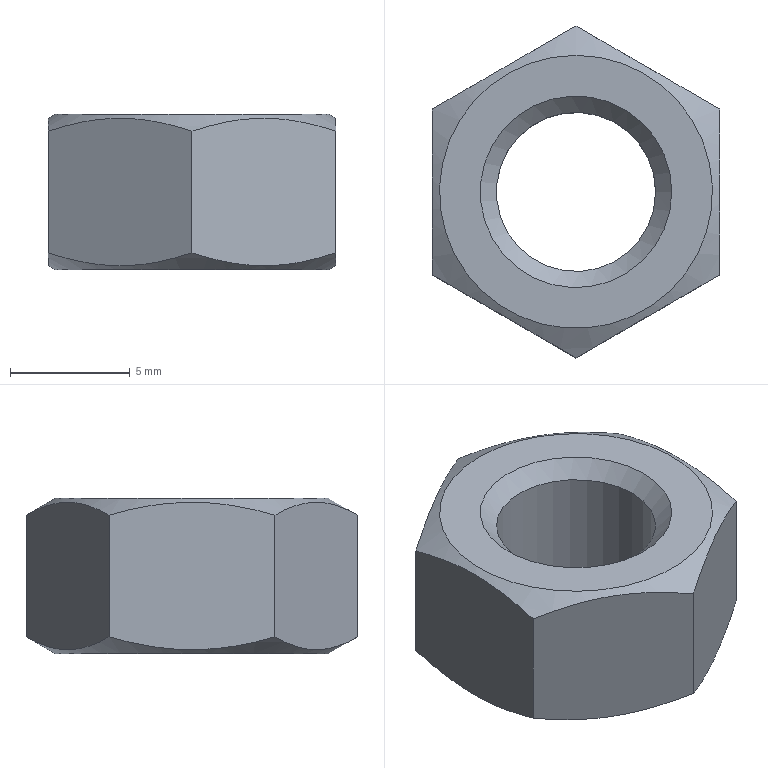Part | STEP file | Гайка М8-6H ГОСТ 15521-70 | 1 solid | 13 faces | box 12 x 13.856 x 6.5 mm | volume 565.148 mm3 | plane 8 | cone 4 | cylinder 1 | commonest cylinder face diameters 6.647 x1
STEP:
#1=CARTESIAN_POINT('',(0.,5.7,0.));
#2=VERTEX_POINT('',#1);
#3=CARTESIAN_POINT('',(0.,0.,0.));
#4=DIRECTION('',(0.,0.,-1.));
#5=DIRECTION('',(0.,1.,0.));
#6=AXIS2_PLACEMENT_3D('',#3,#4,#5);
#7=CIRCLE('',#6,5.7);
#8=EDGE_CURVE('',#2,#2,#7,.T.);
#9=ORIENTED_EDGE('',*,*,#8,.T.);
#10=EDGE_LOOP('',(#9));
#11=FACE_BOUND('',#10,.T.);
#12=CARTESIAN_POINT('',(4.,0.,0.));
#13=VERTEX_POINT('',#12);
#14=CARTESIAN_POINT('',(0.,0.,0.));
#15=DIRECTION('',(0.,0.,1.));
#16=DIRECTION('',(1.,0.,0.));
#17=AXIS2_PLACEMENT_3D('',#14,#15,#16);
#18=CIRCLE('',#17,4.);
#19=EDGE_CURVE('',#13,#13,#18,.T.);
#20=ORIENTED_EDGE('',*,*,#19,.T.);
#21=EDGE_LOOP('',(#20));
#22=FACE_BOUND('',#21,.T.);
#23=CARTESIAN_POINT('',(0.,0.,0.));
#24=DIRECTION('',(0.,0.,1.));
#25=DIRECTION('',(1.,0.,0.));
#26=AXIS2_PLACEMENT_3D('',#23,#24,#25);
#27=PLANE('',#26);
#28=ADVANCED_FACE('',(#11,#22),#27,.F.);
#29=CARTESIAN_POINT('',(-6.,3.464,0.7091));
#30=VERTEX_POINT('',#29);
#31=CARTESIAN_POINT('',(-6.,-3.464,0.7091));
#32=VERTEX_POINT('',#31);
#33=CARTESIAN_POINT('',(-6.,3.464,0.7091));
#34=CARTESIAN_POINT('',(-6.,3.44,0.7022));
#35=CARTESIAN_POINT('',(-6.,3.392,0.6884));
#36=CARTESIAN_POINT('',(-6.,3.319,0.6679));
#37=CARTESIAN_POINT('',(-6.,3.262,0.6521));
#38=CARTESIAN_POINT('',(-6.,3.212,0.6384));
#39=CARTESIAN_POINT('',(-6.,3.161,0.6244));
#40=CARTESIAN_POINT('',(-6.,3.081,0.6031));
#41=CARTESIAN_POINT('',(-6.,2.98,0.5769));
#42=CARTESIAN_POINT('',(-6.,2.867,0.5481));
#43=CARTESIAN_POINT('',(-6.,2.756,0.5211));
#44=CARTESIAN_POINT('',(-6.,2.667,0.4999));
#45=CARTESIAN_POINT('',(-6.,2.597,0.4838));
#46=CARTESIAN_POINT('',(-6.,2.519,0.4659));
#47=CARTESIAN_POINT('',(-6.,2.411,0.4423));
#48=CARTESIAN_POINT('',(-6.,2.271,0.4128));
#49=CARTESIAN_POINT('',(-6.,2.118,0.3823));
#50=CARTESIAN_POINT('',(-6.,1.93,0.3475));
#51=CARTESIAN_POINT('',(-6.,1.792,0.3241));
#52=CARTESIAN_POINT('',(-6.,1.624,0.2976));
#53=CARTESIAN_POINT('',(-6.,1.448,0.2716));
#54=CARTESIAN_POINT('',(-6.,1.203,0.2413));
#55=CARTESIAN_POINT('',(-6.,0.9715,0.2176));
#56=CARTESIAN_POINT('',(-6.,0.8175,0.2049));
#57=CARTESIAN_POINT('',(-6.,0.6729,0.1947));
#58=CARTESIAN_POINT('',(-6.,0.528,0.186));
#59=CARTESIAN_POINT('',(-6.,0.3241,0.1775));
#60=CARTESIAN_POINT('',(-6.,0.1444,0.1738));
#61=CARTESIAN_POINT('',(-6.,0.005553,0.173));
#62=CARTESIAN_POINT('',(-6.,-0.1288,0.1736));
#63=CARTESIAN_POINT('',(-6.,-0.2398,0.1757));
#64=CARTESIAN_POINT('',(-6.,-0.3697,0.1796));
#65=CARTESIAN_POINT('',(-6.,-0.4967,0.1846));
#66=CARTESIAN_POINT('',(-6.,-0.6724,0.1943));
#67=CARTESIAN_POINT('',(-6.,-0.8597,0.208));
#68=CARTESIAN_POINT('',(-6.,-1.046,0.2249));
#69=CARTESIAN_POINT('',(-6.,-1.17,0.2382));
#70=CARTESIAN_POINT('',(-6.,-1.292,0.2525));
#71=CARTESIAN_POINT('',(-6.,-1.414,0.2676));
#72=CARTESIAN_POINT('',(-6.,-1.595,0.293));
#73=CARTESIAN_POINT('',(-6.,-1.774,0.321));
#74=CARTESIAN_POINT('',(-6.,-1.901,0.3428));
#75=CARTESIAN_POINT('',(-6.,-2.018,0.3638));
#76=CARTESIAN_POINT('',(-6.,-2.134,0.3855));
#77=CARTESIAN_POINT('',(-6.,-2.299,0.4185));
#78=CARTESIAN_POINT('',(-6.,-2.471,0.455));
#79=CARTESIAN_POINT('',(-6.,-2.64,0.4933));
#80=CARTESIAN_POINT('',(-6.,-2.785,0.528));
#81=CARTESIAN_POINT('',(-6.,-2.896,0.5556));
#82=CARTESIAN_POINT('',(-6.,-3.007,0.5836));
#83=CARTESIAN_POINT('',(-6.,-3.138,0.6181));
#84=CARTESIAN_POINT('',(-6.,-3.294,0.6607));
#85=CARTESIAN_POINT('',(-6.,-3.403,0.6914));
#86=CARTESIAN_POINT('',(-6.,-3.457,0.707));
#87=CARTESIAN_POINT('',(-6.,-3.464,0.7091));
#88=B_SPLINE_CURVE_WITH_KNOTS('',3,(#33,#34,#35,#36,#37,#38,#39,#40,#41,#42,#43,#44,#45,#46,#47,#48,#49,#50,#51,#52,#53,#54,#55,#56,#57,#58,#59,#60,#61,#62,#63,#64,#65,#66,#67,#68,#69,#70,#71,#72,#73,#74,#75,#76,#77,#78,#79,#80,#81,#82,#83,#84,#85,#86,#87),.UNSPECIFIED.,.F.,.F.,(4,1,1,1,1,1,1,1,1,1,1,1,1,1,1,1,1,1,1,1,1,1,1,1,1,1,1,1,1,1,1,1,1,1,1,1,1,1,1,1,1,1,1,1,1,1,1,1,1,1,1,1,4),(0.,0.01059,0.02135,0.03227,0.03583,0.04354,0.05498,0.07113,0.0878,0.105,0.1195,0.127,0.1355,0.154,0.1738,0.1965,0.2208,0.2552,0.2563,0.2931,0.3312,0.3616,0.3923,0.3971,0.4234,0.4542,0.4842,0.5,0.5134,0.5414,0.5473,0.5689,0.5957,0.6224,0.649,0.6754,0.6755,0.7016,0.7277,0.7534,0.779,0.7826,0.8042,0.8294,0.8542,0.8789,0.9033,0.918,0.9277,0.9518,0.976,0.9967,1.),.UNSPECIFIED.);
#89=EDGE_CURVE('',#30,#32,#88,.T.);
#90=ORIENTED_EDGE('',*,*,#89,.T.);
#91=CARTESIAN_POINT('',(-6.,-3.464,5.791));
#92=VERTEX_POINT('',#91);
#93=CARTESIAN_POINT('',(-6.,-3.464,0.7091));
#94=DIRECTION('',(0.,0.,1.));
#95=VECTOR('',#94,1.);
#96=LINE('',#93,#95);
#97=EDGE_CURVE('',#32,#92,#96,.T.);
#98=ORIENTED_EDGE('',*,*,#97,.T.);
#99=CARTESIAN_POINT('',(-6.,3.464,5.791));
#100=VERTEX_POINT('',#99);
#101=CARTESIAN_POINT('',(-6.,-3.464,5.791));
#102=CARTESIAN_POINT('',(-6.,-3.44,5.798));
#103=CARTESIAN_POINT('',(-6.,-3.392,5.812));
#104=CARTESIAN_POINT('',(-6.,-3.319,5.832));
#105=CARTESIAN_POINT('',(-6.,-3.262,5.848));
#106=CARTESIAN_POINT('',(-6.,-3.212,5.862));
#107=CARTESIAN_POINT('',(-6.,-3.161,5.876));
#108=CARTESIAN_POINT('',(-6.,-3.081,5.897));
#109=CARTESIAN_POINT('',(-6.,-2.98,5.923));
#110=CARTESIAN_POINT('',(-6.,-2.867,5.952));
#111=CARTESIAN_POINT('',(-6.,-2.756,5.979));
#112=CARTESIAN_POINT('',(-6.,-2.667,6.));
#113=CARTESIAN_POINT('',(-6.,-2.597,6.016));
#114=CARTESIAN_POINT('',(-6.,-2.519,6.034));
#115=CARTESIAN_POINT('',(-6.,-2.411,6.058));
#116=CARTESIAN_POINT('',(-6.,-2.271,6.087));
#117=CARTESIAN_POINT('',(-6.,-2.118,6.118));
#118=CARTESIAN_POINT('',(-6.,-1.93,6.153));
#119=CARTESIAN_POINT('',(-6.,-1.792,6.176));
#120=CARTESIAN_POINT('',(-6.,-1.624,6.202));
#121=CARTESIAN_POINT('',(-6.,-1.448,6.228));
#122=CARTESIAN_POINT('',(-6.,-1.203,6.259));
#123=CARTESIAN_POINT('',(-6.,-0.9715,6.282));
#124=CARTESIAN_POINT('',(-6.,-0.8175,6.295));
#125=CARTESIAN_POINT('',(-6.,-0.6729,6.305));
#126=CARTESIAN_POINT('',(-6.,-0.528,6.314));
#127=CARTESIAN_POINT('',(-6.,-0.3241,6.322));
#128=CARTESIAN_POINT('',(-6.,-0.1444,6.326));
#129=CARTESIAN_POINT('',(-6.,-0.005553,6.327));
#130=CARTESIAN_POINT('',(-6.,0.1288,6.326));
#131=CARTESIAN_POINT('',(-6.,0.2398,6.324));
#132=CARTESIAN_POINT('',(-6.,0.3697,6.32));
#133=CARTESIAN_POINT('',(-6.,0.4967,6.315));
#134=CARTESIAN_POINT('',(-6.,0.6724,6.306));
#135=CARTESIAN_POINT('',(-6.,0.8597,6.292));
#136=CARTESIAN_POINT('',(-6.,1.046,6.275));
#137=CARTESIAN_POINT('',(-6.,1.17,6.262));
#138=CARTESIAN_POINT('',(-6.,1.292,6.248));
#139=CARTESIAN_POINT('',(-6.,1.414,6.232));
#140=CARTESIAN_POINT('',(-6.,1.595,6.207));
#141=CARTESIAN_POINT('',(-6.,1.774,6.179));
#142=CARTESIAN_POINT('',(-6.,1.901,6.157));
#143=CARTESIAN_POINT('',(-6.,2.018,6.136));
#144=CARTESIAN_POINT('',(-6.,2.134,6.114));
#145=CARTESIAN_POINT('',(-6.,2.299,6.082));
#146=CARTESIAN_POINT('',(-6.,2.471,6.045));
#147=CARTESIAN_POINT('',(-6.,2.64,6.007));
#148=CARTESIAN_POINT('',(-6.,2.785,5.972));
#149=CARTESIAN_POINT('',(-6.,2.896,5.944));
#150=CARTESIAN_POINT('',(-6.,3.007,5.916));
#151=CARTESIAN_POINT('',(-6.,3.138,5.882));
#152=CARTESIAN_POINT('',(-6.,3.294,5.839));
#153=CARTESIAN_POINT('',(-6.,3.403,5.809));
#154=CARTESIAN_POINT('',(-6.,3.457,5.793));
#155=CARTESIAN_POINT('',(-6.,3.464,5.791));
#156=B_SPLINE_CURVE_WITH_KNOTS('',3,(#101,#102,#103,#104,#105,#106,#107,#108,#109,#110,#111,#112,#113,#114,#115,#116,#117,#118,#119,#120,#121,#122,#123,#124,#125,#126,#127,#128,#129,#130,#131,#132,#133,#134,#135,#136,#137,#138,#139,#140,#141,#142,#143,#144,#145,#146,#147,#148,#149,#150,#151,#152,#153,#154,#155),.UNSPECIFIED.,.F.,.F.,(4,1,1,1,1,1,1,1,1,1,1,1,1,1,1,1,1,1,1,1,1,1,1,1,1,1,1,1,1,1,1,1,1,1,1,1,1,1,1,1,1,1,1,1,1,1,1,1,1,1,1,1,4),(0.,0.01059,0.02135,0.03227,0.03583,0.04354,0.05498,0.07113,0.0878,0.105,0.1195,0.127,0.1355,0.154,0.1738,0.1965,0.2208,0.2552,0.2563,0.2931,0.3312,0.3616,0.3923,0.3971,0.4234,0.4542,0.4842,0.5,0.5134,0.5414,0.5473,0.5689,0.5957,0.6224,0.649,0.6754,0.6755,0.7016,0.7277,0.7534,0.779,0.7826,0.8042,0.8294,0.8542,0.8789,0.9033,0.918,0.9277,0.9518,0.976,0.9967,1.),.UNSPECIFIED.);
#157=EDGE_CURVE('',#92,#100,#156,.T.);
#158=ORIENTED_EDGE('',*,*,#157,.T.);
#159=CARTESIAN_POINT('',(-6.,3.464,0.7091));
#160=DIRECTION('',(0.,0.,1.));
#161=VECTOR('',#160,1.);
#162=LINE('',#159,#161);
#163=EDGE_CURVE('',#30,#100,#162,.T.);
#164=ORIENTED_EDGE('',*,*,#163,.F.);
#165=EDGE_LOOP('',(#90,#98,#158,#164));
#166=FACE_BOUND('',#165,.T.);
#167=CARTESIAN_POINT('',(-6.,3.464,0.));
#168=DIRECTION('',(-1.,0.,0.));
#169=DIRECTION('',(0.,-1.,0.));
#170=AXIS2_PLACEMENT_3D('',#167,#168,#169);
#171=PLANE('',#170);
#172=ADVANCED_FACE('',(#166),#171,.T.);
#173=CARTESIAN_POINT('',(0.,6.928,0.7091));
#174=VERTEX_POINT('',#173);
#175=CARTESIAN_POINT('',(0.,6.928,0.7091));
#176=CARTESIAN_POINT('',(-0.02065,6.916,0.7022));
#177=CARTESIAN_POINT('',(-0.06231,6.892,0.6884));
#178=CARTESIAN_POINT('',(-0.1254,6.856,0.6679));
#179=CARTESIAN_POINT('',(-0.1899,6.819,0.6473));
#180=CARTESIAN_POINT('',(-0.2557,6.781,0.6266));
#181=CARTESIAN_POINT('',(-0.332,6.737,0.6031));
#182=CARTESIAN_POINT('',(-0.419,6.686,0.5769));
#183=CARTESIAN_POINT('',(-0.5174,6.629,0.5481));
#184=CARTESIAN_POINT('',(-0.6129,6.574,0.5211));
#185=CARTESIAN_POINT('',(-0.7071,6.52,0.4954));
#186=CARTESIAN_POINT('',(-0.8041,6.464,0.4697));
#187=CARTESIAN_POINT('',(-0.9117,6.402,0.4423));
#188=CARTESIAN_POINT('',(-1.033,6.332,0.4128));
#189=CARTESIAN_POINT('',(-1.166,6.255,0.3823));
#190=CARTESIAN_POINT('',(-1.331,6.16,0.347));
#191=CARTESIAN_POINT('',(-1.524,6.048,0.3093));
#192=CARTESIAN_POINT('',(-1.746,5.92,0.2716));
#193=CARTESIAN_POINT('',(-1.958,5.798,0.2413));
#194=CARTESIAN_POINT('',(-2.159,5.682,0.2176));
#195=CARTESIAN_POINT('',(-2.345,5.574,0.1999));
#196=CARTESIAN_POINT('',(-2.533,5.466,0.1864));
#197=CARTESIAN_POINT('',(-2.719,5.358,0.1775));
#198=CARTESIAN_POINT('',(-2.875,5.268,0.1738));
#199=CARTESIAN_POINT('',(-2.995,5.199,0.173));
#200=CARTESIAN_POINT('',(-3.112,5.132,0.1736));
#201=CARTESIAN_POINT('',(-3.251,5.051,0.1766));
#202=CARTESIAN_POINT('',(-3.418,4.955,0.1838));
#203=CARTESIAN_POINT('',(-3.582,4.86,0.1943));
#204=CARTESIAN_POINT('',(-3.745,4.766,0.208));
#205=CARTESIAN_POINT('',(-3.906,4.673,0.2249));
#206=CARTESIAN_POINT('',(-4.066,4.581,0.2448));
#207=CARTESIAN_POINT('',(-4.224,4.489,0.2676));
#208=CARTESIAN_POINT('',(-4.381,4.399,0.293));
#209=CARTESIAN_POINT('',(-4.536,4.309,0.321));
#210=CARTESIAN_POINT('',(-4.69,4.221,0.3513));
#211=CARTESIAN_POINT('',(-4.841,4.133,0.3839));
#212=CARTESIAN_POINT('',(-4.991,4.047,0.4185));
#213=CARTESIAN_POINT('',(-5.14,3.961,0.455));
#214=CARTESIAN_POINT('',(-5.286,3.876,0.4933));
#215=CARTESIAN_POINT('',(-5.431,3.792,0.5333));
#216=CARTESIAN_POINT('',(-5.575,3.709,0.5749));
#217=CARTESIAN_POINT('',(-5.718,3.627,0.6181));
#218=CARTESIAN_POINT('',(-5.859,3.545,0.6627));
#219=CARTESIAN_POINT('',(-5.953,3.491,0.6935));
#220=CARTESIAN_POINT('',(-6.,3.464,0.7091));
#221=B_SPLINE_CURVE_WITH_KNOTS('',3,(#175,#176,#177,#178,#179,#180,#181,#182,#183,#184,#185,#186,#187,#188,#189,#190,#191,#192,#193,#194,#195,#196,#197,#198,#199,#200,#201,#202,#203,#204,#205,#206,#207,#208,#209,#210,#211,#212,#213,#214,#215,#216,#217,#218,#219,#220),.UNSPECIFIED.,.F.,.F.,(4,1,1,1,1,1,1,1,1,1,1,1,1,1,1,1,1,1,1,1,1,1,1,1,1,1,1,1,1,1,1,1,1,1,1,1,1,1,1,1,1,1,1,4),(0.,0.01059,0.02135,0.03227,0.04354,0.05498,0.07113,0.0878,0.105,0.1195,0.1355,0.154,0.1738,0.1965,0.2208,0.2563,0.2931,0.3312,0.3616,0.3923,0.4234,0.4542,0.4842,0.5,0.5134,0.5414,0.5689,0.5957,0.6224,0.649,0.6754,0.7016,0.7277,0.7534,0.779,0.8042,0.8294,0.8542,0.8789,0.9033,0.9277,0.9518,0.976,1.),.UNSPECIFIED.);
#222=EDGE_CURVE('',#174,#30,#221,.T.);
#223=ORIENTED_EDGE('',*,*,#222,.T.);
#224=ORIENTED_EDGE('',*,*,#163,.T.);
#225=CARTESIAN_POINT('',(0.,6.928,5.791));
#226=VERTEX_POINT('',#225);
#227=CARTESIAN_POINT('',(-6.,3.464,5.791));
#228=CARTESIAN_POINT('',(-5.979,3.476,5.798));
#229=CARTESIAN_POINT('',(-5.938,3.5,5.812));
#230=CARTESIAN_POINT('',(-5.875,3.536,5.832));
#231=CARTESIAN_POINT('',(-5.81,3.574,5.853));
#232=CARTESIAN_POINT('',(-5.744,3.612,5.873));
#233=CARTESIAN_POINT('',(-5.668,3.656,5.897));
#234=CARTESIAN_POINT('',(-5.581,3.706,5.923));
#235=CARTESIAN_POINT('',(-5.483,3.763,5.952));
#236=CARTESIAN_POINT('',(-5.387,3.818,5.979));
#237=CARTESIAN_POINT('',(-5.293,3.872,6.005));
#238=CARTESIAN_POINT('',(-5.196,3.928,6.03));
#239=CARTESIAN_POINT('',(-5.088,3.99,6.058));
#240=CARTESIAN_POINT('',(-4.967,4.06,6.087));
#241=CARTESIAN_POINT('',(-4.834,4.137,6.118));
#242=CARTESIAN_POINT('',(-4.669,4.232,6.153));
#243=CARTESIAN_POINT('',(-4.476,4.344,6.191));
#244=CARTESIAN_POINT('',(-4.254,4.472,6.228));
#245=CARTESIAN_POINT('',(-4.042,4.595,6.259));
#246=CARTESIAN_POINT('',(-3.841,4.71,6.282));
#247=CARTESIAN_POINT('',(-3.655,4.818,6.3));
#248=CARTESIAN_POINT('',(-3.467,4.927,6.314));
#249=CARTESIAN_POINT('',(-3.281,5.034,6.322));
#250=CARTESIAN_POINT('',(-3.125,5.124,6.326));
#251=CARTESIAN_POINT('',(-3.005,5.193,6.327));
#252=CARTESIAN_POINT('',(-2.888,5.261,6.326));
#253=CARTESIAN_POINT('',(-2.749,5.341,6.323));
#254=CARTESIAN_POINT('',(-2.582,5.438,6.316));
#255=CARTESIAN_POINT('',(-2.418,5.532,6.306));
#256=CARTESIAN_POINT('',(-2.255,5.626,6.292));
#257=CARTESIAN_POINT('',(-2.094,5.719,6.275));
#258=CARTESIAN_POINT('',(-1.934,5.811,6.255));
#259=CARTESIAN_POINT('',(-1.776,5.903,6.232));
#260=CARTESIAN_POINT('',(-1.619,5.994,6.207));
#261=CARTESIAN_POINT('',(-1.464,6.083,6.179));
#262=CARTESIAN_POINT('',(-1.31,6.172,6.149));
#263=CARTESIAN_POINT('',(-1.159,6.259,6.116));
#264=CARTESIAN_POINT('',(-1.009,6.346,6.082));
#265=CARTESIAN_POINT('',(-0.8604,6.431,6.045));
#266=CARTESIAN_POINT('',(-0.7138,6.516,6.007));
#267=CARTESIAN_POINT('',(-0.5687,6.6,5.967));
#268=CARTESIAN_POINT('',(-0.425,6.683,5.925));
#269=CARTESIAN_POINT('',(-0.2824,6.765,5.882));
#270=CARTESIAN_POINT('',(-0.1408,6.847,5.837));
#271=CARTESIAN_POINT('',(-0.04683,6.901,5.807));
#272=CARTESIAN_POINT('',(0.000000002,6.928,5.791));
#273=B_SPLINE_CURVE_WITH_KNOTS('',3,(#227,#228,#229,#230,#231,#232,#233,#234,#235,#236,#237,#238,#239,#240,#241,#242,#243,#244,#245,#246,#247,#248,#249,#250,#251,#252,#253,#254,#255,#256,#257,#258,#259,#260,#261,#262,#263,#264,#265,#266,#267,#268,#269,#270,#271,#272),.UNSPECIFIED.,.F.,.F.,(4,1,1,1,1,1,1,1,1,1,1,1,1,1,1,1,1,1,1,1,1,1,1,1,1,1,1,1,1,1,1,1,1,1,1,1,1,1,1,1,1,1,1,4),(0.,0.01059,0.02135,0.03227,0.04354,0.05498,0.07113,0.0878,0.105,0.1195,0.1355,0.154,0.1738,0.1965,0.2208,0.2563,0.2931,0.3312,0.3616,0.3923,0.4234,0.4542,0.4842,0.5,0.5134,0.5414,0.5689,0.5957,0.6224,0.649,0.6754,0.7016,0.7277,0.7534,0.779,0.8042,0.8294,0.8542,0.8789,0.9033,0.9277,0.9518,0.976,1.),.UNSPECIFIED.);
#274=EDGE_CURVE('',#100,#226,#273,.T.);
#275=ORIENTED_EDGE('',*,*,#274,.T.);
#276=CARTESIAN_POINT('',(0.,6.928,0.7091));
#277=DIRECTION('',(0.,0.,1.));
#278=VECTOR('',#277,1.);
#279=LINE('',#276,#278);
#280=EDGE_CURVE('',#174,#226,#279,.T.);
#281=ORIENTED_EDGE('',*,*,#280,.F.);
#282=EDGE_LOOP('',(#223,#224,#275,#281));
#283=FACE_BOUND('',#282,.T.);
#284=CARTESIAN_POINT('',(0.,6.928,0.));
#285=DIRECTION('',(-0.5,0.866,0.));
#286=DIRECTION('',(-0.866,-0.5,0.));
#287=AXIS2_PLACEMENT_3D('',#284,#285,#286);
#288=PLANE('',#287);
#289=ADVANCED_FACE('',(#283),#288,.T.);
#290=CARTESIAN_POINT('',(6.,3.464,0.7091));
#291=VERTEX_POINT('',#290);
#292=CARTESIAN_POINT('',(6.,3.464,0.7091));
#293=CARTESIAN_POINT('',(5.979,3.476,0.7022));
#294=CARTESIAN_POINT('',(5.938,3.5,0.6884));
#295=CARTESIAN_POINT('',(5.875,3.536,0.6679));
#296=CARTESIAN_POINT('',(5.81,3.574,0.6473));
#297=CARTESIAN_POINT('',(5.744,3.612,0.6266));
#298=CARTESIAN_POINT('',(5.668,3.656,0.6031));
#299=CARTESIAN_POINT('',(5.581,3.706,0.5769));
#300=CARTESIAN_POINT('',(5.483,3.763,0.5481));
#301=CARTESIAN_POINT('',(5.387,3.818,0.5211));
#302=CARTESIAN_POINT('',(5.293,3.872,0.4954));
#303=CARTESIAN_POINT('',(5.196,3.928,0.4697));
#304=CARTESIAN_POINT('',(5.088,3.99,0.4423));
#305=CARTESIAN_POINT('',(4.967,4.06,0.4128));
#306=CARTESIAN_POINT('',(4.834,4.137,0.3823));
#307=CARTESIAN_POINT('',(4.669,4.232,0.347));
#308=CARTESIAN_POINT('',(4.476,4.344,0.3093));
#309=CARTESIAN_POINT('',(4.254,4.472,0.2716));
#310=CARTESIAN_POINT('',(4.042,4.595,0.2413));
#311=CARTESIAN_POINT('',(3.841,4.71,0.2176));
#312=CARTESIAN_POINT('',(3.655,4.818,0.1999));
#313=CARTESIAN_POINT('',(3.467,4.927,0.1864));
#314=CARTESIAN_POINT('',(3.281,5.034,0.1775));
#315=CARTESIAN_POINT('',(3.125,5.124,0.1738));
#316=CARTESIAN_POINT('',(3.005,5.193,0.173));
#317=CARTESIAN_POINT('',(2.888,5.261,0.1736));
#318=CARTESIAN_POINT('',(2.749,5.341,0.1766));
#319=CARTESIAN_POINT('',(2.582,5.438,0.1838));
#320=CARTESIAN_POINT('',(2.418,5.532,0.1943));
#321=CARTESIAN_POINT('',(2.255,5.626,0.208));
#322=CARTESIAN_POINT('',(2.094,5.719,0.2249));
#323=CARTESIAN_POINT('',(1.934,5.811,0.2448));
#324=CARTESIAN_POINT('',(1.776,5.903,0.2676));
#325=CARTESIAN_POINT('',(1.619,5.994,0.293));
#326=CARTESIAN_POINT('',(1.464,6.083,0.321));
#327=CARTESIAN_POINT('',(1.31,6.172,0.3513));
#328=CARTESIAN_POINT('',(1.159,6.259,0.3839));
#329=CARTESIAN_POINT('',(1.009,6.346,0.4185));
#330=CARTESIAN_POINT('',(0.8604,6.431,0.455));
#331=CARTESIAN_POINT('',(0.7138,6.516,0.4933));
#332=CARTESIAN_POINT('',(0.5687,6.6,0.5333));
#333=CARTESIAN_POINT('',(0.425,6.683,0.5749));
#334=CARTESIAN_POINT('',(0.2824,6.765,0.6181));
#335=CARTESIAN_POINT('',(0.1408,6.847,0.6627));
#336=CARTESIAN_POINT('',(0.04683,6.901,0.6935));
#337=CARTESIAN_POINT('',(0.000000002,6.928,0.7091));
#338=B_SPLINE_CURVE_WITH_KNOTS('',3,(#292,#293,#294,#295,#296,#297,#298,#299,#300,#301,#302,#303,#304,#305,#306,#307,#308,#309,#310,#311,#312,#313,#314,#315,#316,#317,#318,#319,#320,#321,#322,#323,#324,#325,#326,#327,#328,#329,#330,#331,#332,#333,#334,#335,#336,#337),.UNSPECIFIED.,.F.,.F.,(4,1,1,1,1,1,1,1,1,1,1,1,1,1,1,1,1,1,1,1,1,1,1,1,1,1,1,1,1,1,1,1,1,1,1,1,1,1,1,1,1,1,1,4),(0.,0.01059,0.02135,0.03227,0.04354,0.05498,0.07113,0.0878,0.105,0.1195,0.1355,0.154,0.1738,0.1965,0.2208,0.2563,0.2931,0.3312,0.3616,0.3923,0.4234,0.4542,0.4842,0.5,0.5134,0.5414,0.5689,0.5957,0.6224,0.649,0.6754,0.7016,0.7277,0.7534,0.779,0.8042,0.8294,0.8542,0.8789,0.9033,0.9277,0.9518,0.976,1.),.UNSPECIFIED.);
#339=EDGE_CURVE('',#291,#174,#338,.T.);
#340=ORIENTED_EDGE('',*,*,#339,.T.);
#341=ORIENTED_EDGE('',*,*,#280,.T.);
#342=CARTESIAN_POINT('',(6.,3.464,5.791));
#343=VERTEX_POINT('',#342);
#344=CARTESIAN_POINT('',(0.,6.928,5.791));
#345=CARTESIAN_POINT('',(0.02065,6.916,5.798));
#346=CARTESIAN_POINT('',(0.06231,6.892,5.812));
#347=CARTESIAN_POINT('',(0.1254,6.856,5.832));
#348=CARTESIAN_POINT('',(0.1899,6.819,5.853));
#349=CARTESIAN_POINT('',(0.2557,6.781,5.873));
#350=CARTESIAN_POINT('',(0.332,6.737,5.897));
#351=CARTESIAN_POINT('',(0.419,6.686,5.923));
#352=CARTESIAN_POINT('',(0.5174,6.629,5.952));
#353=CARTESIAN_POINT('',(0.6129,6.574,5.979));
#354=CARTESIAN_POINT('',(0.7071,6.52,6.005));
#355=CARTESIAN_POINT('',(0.8041,6.464,6.03));
#356=CARTESIAN_POINT('',(0.9117,6.402,6.058));
#357=CARTESIAN_POINT('',(1.033,6.332,6.087));
#358=CARTESIAN_POINT('',(1.166,6.255,6.118));
#359=CARTESIAN_POINT('',(1.331,6.16,6.153));
#360=CARTESIAN_POINT('',(1.524,6.048,6.191));
#361=CARTESIAN_POINT('',(1.746,5.92,6.228));
#362=CARTESIAN_POINT('',(1.958,5.798,6.259));
#363=CARTESIAN_POINT('',(2.159,5.682,6.282));
#364=CARTESIAN_POINT('',(2.345,5.574,6.3));
#365=CARTESIAN_POINT('',(2.533,5.466,6.314));
#366=CARTESIAN_POINT('',(2.719,5.358,6.322));
#367=CARTESIAN_POINT('',(2.875,5.268,6.326));
#368=CARTESIAN_POINT('',(2.995,5.199,6.327));
#369=CARTESIAN_POINT('',(3.112,5.132,6.326));
#370=CARTESIAN_POINT('',(3.251,5.051,6.323));
#371=CARTESIAN_POINT('',(3.418,4.955,6.316));
#372=CARTESIAN_POINT('',(3.582,4.86,6.306));
#373=CARTESIAN_POINT('',(3.745,4.766,6.292));
#374=CARTESIAN_POINT('',(3.906,4.673,6.275));
#375=CARTESIAN_POINT('',(4.066,4.581,6.255));
#376=CARTESIAN_POINT('',(4.224,4.489,6.232));
#377=CARTESIAN_POINT('',(4.381,4.399,6.207));
#378=CARTESIAN_POINT('',(4.536,4.309,6.179));
#379=CARTESIAN_POINT('',(4.69,4.221,6.149));
#380=CARTESIAN_POINT('',(4.841,4.133,6.116));
#381=CARTESIAN_POINT('',(4.991,4.047,6.082));
#382=CARTESIAN_POINT('',(5.14,3.961,6.045));
#383=CARTESIAN_POINT('',(5.286,3.876,6.007));
#384=CARTESIAN_POINT('',(5.431,3.792,5.967));
#385=CARTESIAN_POINT('',(5.575,3.709,5.925));
#386=CARTESIAN_POINT('',(5.718,3.627,5.882));
#387=CARTESIAN_POINT('',(5.859,3.545,5.837));
#388=CARTESIAN_POINT('',(5.953,3.491,5.807));
#389=CARTESIAN_POINT('',(6.,3.464,5.791));
#390=B_SPLINE_CURVE_WITH_KNOTS('',3,(#344,#345,#346,#347,#348,#349,#350,#351,#352,#353,#354,#355,#356,#357,#358,#359,#360,#361,#362,#363,#364,#365,#366,#367,#368,#369,#370,#371,#372,#373,#374,#375,#376,#377,#378,#379,#380,#381,#382,#383,#384,#385,#386,#387,#388,#389),.UNSPECIFIED.,.F.,.F.,(4,1,1,1,1,1,1,1,1,1,1,1,1,1,1,1,1,1,1,1,1,1,1,1,1,1,1,1,1,1,1,1,1,1,1,1,1,1,1,1,1,1,1,4),(0.,0.01059,0.02135,0.03227,0.04354,0.05498,0.07113,0.0878,0.105,0.1195,0.1355,0.154,0.1738,0.1965,0.2208,0.2563,0.2931,0.3312,0.3616,0.3923,0.4234,0.4542,0.4842,0.5,0.5134,0.5414,0.5689,0.5957,0.6224,0.649,0.6754,0.7016,0.7277,0.7534,0.779,0.8042,0.8294,0.8542,0.8789,0.9033,0.9277,0.9518,0.976,1.),.UNSPECIFIED.);
#391=EDGE_CURVE('',#226,#343,#390,.T.);
#392=ORIENTED_EDGE('',*,*,#391,.T.);
#393=CARTESIAN_POINT('',(6.,3.464,0.7091));
#394=DIRECTION('',(0.,0.,1.));
#395=VECTOR('',#394,1.);
#396=LINE('',#393,#395);
#397=EDGE_CURVE('',#291,#343,#396,.T.);
#398=ORIENTED_EDGE('',*,*,#397,.F.);
#399=EDGE_LOOP('',(#340,#341,#392,#398));
#400=FACE_BOUND('',#399,.T.);
#401=CARTESIAN_POINT('',(6.,3.464,0.));
#402=DIRECTION('',(0.5,0.866,0.));
#403=DIRECTION('',(-0.866,0.5,0.));
#404=AXIS2_PLACEMENT_3D('',#401,#402,#403);
#405=PLANE('',#404);
#406=ADVANCED_FACE('',(#400),#405,.T.);
#407=CARTESIAN_POINT('',(6.,-3.464,0.7091));
#408=VERTEX_POINT('',#407);
#409=CARTESIAN_POINT('',(6.,-3.464,0.7091));
#410=CARTESIAN_POINT('',(6.,-3.44,0.7022));
#411=CARTESIAN_POINT('',(6.,-3.392,0.6884));
#412=CARTESIAN_POINT('',(6.,-3.319,0.6679));
#413=CARTESIAN_POINT('',(6.,-3.262,0.6521));
#414=CARTESIAN_POINT('',(6.,-3.212,0.6384));
#415=CARTESIAN_POINT('',(6.,-3.161,0.6244));
#416=CARTESIAN_POINT('',(6.,-3.081,0.6031));
#417=CARTESIAN_POINT('',(6.,-2.98,0.5769));
#418=CARTESIAN_POINT('',(6.,-2.867,0.5481));
#419=CARTESIAN_POINT('',(6.,-2.756,0.5211));
#420=CARTESIAN_POINT('',(6.,-2.667,0.4999));
#421=CARTESIAN_POINT('',(6.,-2.597,0.4838));
#422=CARTESIAN_POINT('',(6.,-2.519,0.4659));
#423=CARTESIAN_POINT('',(6.,-2.411,0.4423));
#424=CARTESIAN_POINT('',(6.,-2.271,0.4128));
#425=CARTESIAN_POINT('',(6.,-2.118,0.3823));
#426=CARTESIAN_POINT('',(6.,-1.93,0.3475));
#427=CARTESIAN_POINT('',(6.,-1.792,0.3241));
#428=CARTESIAN_POINT('',(6.,-1.624,0.2976));
#429=CARTESIAN_POINT('',(6.,-1.448,0.2716));
#430=CARTESIAN_POINT('',(6.,-1.203,0.2413));
#431=CARTESIAN_POINT('',(6.,-0.9715,0.2176));
#432=CARTESIAN_POINT('',(6.,-0.8175,0.2049));
#433=CARTESIAN_POINT('',(6.,-0.6729,0.1947));
#434=CARTESIAN_POINT('',(6.,-0.528,0.186));
#435=CARTESIAN_POINT('',(6.,-0.3241,0.1775));
#436=CARTESIAN_POINT('',(6.,-0.1444,0.1738));
#437=CARTESIAN_POINT('',(6.,-0.005553,0.173));
#438=CARTESIAN_POINT('',(6.,0.1288,0.1736));
#439=CARTESIAN_POINT('',(6.,0.2398,0.1757));
#440=CARTESIAN_POINT('',(6.,0.3697,0.1796));
#441=CARTESIAN_POINT('',(6.,0.4967,0.1846));
#442=CARTESIAN_POINT('',(6.,0.6724,0.1943));
#443=CARTESIAN_POINT('',(6.,0.8597,0.208));
#444=CARTESIAN_POINT('',(6.,1.046,0.2249));
#445=CARTESIAN_POINT('',(6.,1.17,0.2382));
#446=CARTESIAN_POINT('',(6.,1.292,0.2525));
#447=CARTESIAN_POINT('',(6.,1.414,0.2676));
#448=CARTESIAN_POINT('',(6.,1.595,0.293));
#449=CARTESIAN_POINT('',(6.,1.774,0.321));
#450=CARTESIAN_POINT('',(6.,1.901,0.3428));
#451=CARTESIAN_POINT('',(6.,2.018,0.3638));
#452=CARTESIAN_POINT('',(6.,2.134,0.3855));
#453=CARTESIAN_POINT('',(6.,2.299,0.4185));
#454=CARTESIAN_POINT('',(6.,2.471,0.455));
#455=CARTESIAN_POINT('',(6.,2.64,0.4933));
#456=CARTESIAN_POINT('',(6.,2.785,0.528));
#457=CARTESIAN_POINT('',(6.,2.896,0.5556));
#458=CARTESIAN_POINT('',(6.,3.007,0.5836));
#459=CARTESIAN_POINT('',(6.,3.138,0.6181));
#460=CARTESIAN_POINT('',(6.,3.294,0.6607));
#461=CARTESIAN_POINT('',(6.,3.403,0.6914));
#462=CARTESIAN_POINT('',(6.,3.457,0.707));
#463=CARTESIAN_POINT('',(6.,3.464,0.7091));
#464=B_SPLINE_CURVE_WITH_KNOTS('',3,(#409,#410,#411,#412,#413,#414,#415,#416,#417,#418,#419,#420,#421,#422,#423,#424,#425,#426,#427,#428,#429,#430,#431,#432,#433,#434,#435,#436,#437,#438,#439,#440,#441,#442,#443,#444,#445,#446,#447,#448,#449,#450,#451,#452,#453,#454,#455,#456,#457,#458,#459,#460,#461,#462,#463),.UNSPECIFIED.,.F.,.F.,(4,1,1,1,1,1,1,1,1,1,1,1,1,1,1,1,1,1,1,1,1,1,1,1,1,1,1,1,1,1,1,1,1,1,1,1,1,1,1,1,1,1,1,1,1,1,1,1,1,1,1,1,4),(0.,0.01059,0.02135,0.03227,0.03583,0.04354,0.05498,0.07113,0.0878,0.105,0.1195,0.127,0.1355,0.154,0.1738,0.1965,0.2208,0.2552,0.2563,0.2931,0.3312,0.3616,0.3923,0.3971,0.4234,0.4542,0.4842,0.5,0.5134,0.5414,0.5473,0.5689,0.5957,0.6224,0.649,0.6754,0.6755,0.7016,0.7277,0.7534,0.779,0.7826,0.8042,0.8294,0.8542,0.8789,0.9033,0.918,0.9277,0.9518,0.976,0.9967,1.),.UNSPECIFIED.);
#465=EDGE_CURVE('',#408,#291,#464,.T.);
#466=ORIENTED_EDGE('',*,*,#465,.T.);
#467=ORIENTED_EDGE('',*,*,#397,.T.);
#468=CARTESIAN_POINT('',(6.,-3.464,5.791));
#469=VERTEX_POINT('',#468);
#470=CARTESIAN_POINT('',(6.,3.464,5.791));
#471=CARTESIAN_POINT('',(6.,3.44,5.798));
#472=CARTESIAN_POINT('',(6.,3.392,5.812));
#473=CARTESIAN_POINT('',(6.,3.319,5.832));
#474=CARTESIAN_POINT('',(6.,3.262,5.848));
#475=CARTESIAN_POINT('',(6.,3.212,5.862));
#476=CARTESIAN_POINT('',(6.,3.161,5.876));
#477=CARTESIAN_POINT('',(6.,3.081,5.897));
#478=CARTESIAN_POINT('',(6.,2.98,5.923));
#479=CARTESIAN_POINT('',(6.,2.867,5.952));
#480=CARTESIAN_POINT('',(6.,2.756,5.979));
#481=CARTESIAN_POINT('',(6.,2.667,6.));
#482=CARTESIAN_POINT('',(6.,2.597,6.016));
#483=CARTESIAN_POINT('',(6.,2.519,6.034));
#484=CARTESIAN_POINT('',(6.,2.411,6.058));
#485=CARTESIAN_POINT('',(6.,2.271,6.087));
#486=CARTESIAN_POINT('',(6.,2.118,6.118));
#487=CARTESIAN_POINT('',(6.,1.93,6.153));
#488=CARTESIAN_POINT('',(6.,1.792,6.176));
#489=CARTESIAN_POINT('',(6.,1.624,6.202));
#490=CARTESIAN_POINT('',(6.,1.448,6.228));
#491=CARTESIAN_POINT('',(6.,1.203,6.259));
#492=CARTESIAN_POINT('',(6.,0.9715,6.282));
#493=CARTESIAN_POINT('',(6.,0.8175,6.295));
#494=CARTESIAN_POINT('',(6.,0.6729,6.305));
#495=CARTESIAN_POINT('',(6.,0.528,6.314));
#496=CARTESIAN_POINT('',(6.,0.3241,6.322));
#497=CARTESIAN_POINT('',(6.,0.1444,6.326));
#498=CARTESIAN_POINT('',(6.,0.005553,6.327));
#499=CARTESIAN_POINT('',(6.,-0.1288,6.326));
#500=CARTESIAN_POINT('',(6.,-0.2398,6.324));
#501=CARTESIAN_POINT('',(6.,-0.3697,6.32));
#502=CARTESIAN_POINT('',(6.,-0.4967,6.315));
#503=CARTESIAN_POINT('',(6.,-0.6724,6.306));
#504=CARTESIAN_POINT('',(6.,-0.8597,6.292));
#505=CARTESIAN_POINT('',(6.,-1.046,6.275));
#506=CARTESIAN_POINT('',(6.,-1.17,6.262));
#507=CARTESIAN_POINT('',(6.,-1.292,6.248));
#508=CARTESIAN_POINT('',(6.,-1.414,6.232));
#509=CARTESIAN_POINT('',(6.,-1.595,6.207));
#510=CARTESIAN_POINT('',(6.,-1.774,6.179));
#511=CARTESIAN_POINT('',(6.,-1.901,6.157));
#512=CARTESIAN_POINT('',(6.,-2.018,6.136));
#513=CARTESIAN_POINT('',(6.,-2.134,6.114));
#514=CARTESIAN_POINT('',(6.,-2.299,6.082));
#515=CARTESIAN_POINT('',(6.,-2.471,6.045));
#516=CARTESIAN_POINT('',(6.,-2.64,6.007));
#517=CARTESIAN_POINT('',(6.,-2.785,5.972));
#518=CARTESIAN_POINT('',(6.,-2.896,5.944));
#519=CARTESIAN_POINT('',(6.,-3.007,5.916));
#520=CARTESIAN_POINT('',(6.,-3.138,5.882));
#521=CARTESIAN_POINT('',(6.,-3.294,5.839));
#522=CARTESIAN_POINT('',(6.,-3.403,5.809));
#523=CARTESIAN_POINT('',(6.,-3.457,5.793));
#524=CARTESIAN_POINT('',(6.,-3.464,5.791));
#525=B_SPLINE_CURVE_WITH_KNOTS('',3,(#470,#471,#472,#473,#474,#475,#476,#477,#478,#479,#480,#481,#482,#483,#484,#485,#486,#487,#488,#489,#490,#491,#492,#493,#494,#495,#496,#497,#498,#499,#500,#501,#502,#503,#504,#505,#506,#507,#508,#509,#510,#511,#512,#513,#514,#515,#516,#517,#518,#519,#520,#521,#522,#523,#524),.UNSPECIFIED.,.F.,.F.,(4,1,1,1,1,1,1,1,1,1,1,1,1,1,1,1,1,1,1,1,1,1,1,1,1,1,1,1,1,1,1,1,1,1,1,1,1,1,1,1,1,1,1,1,1,1,1,1,1,1,1,1,4),(0.,0.01059,0.02135,0.03227,0.03583,0.04354,0.05498,0.07113,0.0878,0.105,0.1195,0.127,0.1355,0.154,0.1738,0.1965,0.2208,0.2552,0.2563,0.2931,0.3312,0.3616,0.3923,0.3971,0.4234,0.4542,0.4842,0.5,0.5134,0.5414,0.5473,0.5689,0.5957,0.6224,0.649,0.6754,0.6755,0.7016,0.7277,0.7534,0.779,0.7826,0.8042,0.8294,0.8542,0.8789,0.9033,0.918,0.9277,0.9518,0.976,0.9967,1.),.UNSPECIFIED.);
#526=EDGE_CURVE('',#343,#469,#525,.T.);
#527=ORIENTED_EDGE('',*,*,#526,.T.);
#528=CARTESIAN_POINT('',(6.,-3.464,0.7091));
#529=DIRECTION('',(0.,0.,1.));
#530=VECTOR('',#529,1.);
#531=LINE('',#528,#530);
#532=EDGE_CURVE('',#408,#469,#531,.T.);
#533=ORIENTED_EDGE('',*,*,#532,.F.);
#534=EDGE_LOOP('',(#466,#467,#527,#533));
#535=FACE_BOUND('',#534,.T.);
#536=CARTESIAN_POINT('',(6.,-3.464,0.));
#537=DIRECTION('',(1.,0.,0.));
#538=DIRECTION('',(0.,1.,0.));
#539=AXIS2_PLACEMENT_3D('',#536,#537,#538);
#540=PLANE('',#539);
#541=ADVANCED_FACE('',(#535),#540,.T.);
#542=CARTESIAN_POINT('',(0.,-6.928,0.7091));
#543=VERTEX_POINT('',#542);
#544=CARTESIAN_POINT('',(0.,-6.928,0.7091));
#545=CARTESIAN_POINT('',(0.02065,-6.916,0.7022));
#546=CARTESIAN_POINT('',(0.06231,-6.892,0.6884));
#547=CARTESIAN_POINT('',(0.1254,-6.856,0.6679));
#548=CARTESIAN_POINT('',(0.1899,-6.819,0.6473));
#549=CARTESIAN_POINT('',(0.2557,-6.781,0.6266));
#550=CARTESIAN_POINT('',(0.332,-6.737,0.6031));
#551=CARTESIAN_POINT('',(0.419,-6.686,0.5769));
#552=CARTESIAN_POINT('',(0.5174,-6.629,0.5481));
#553=CARTESIAN_POINT('',(0.6129,-6.574,0.5211));
#554=CARTESIAN_POINT('',(0.7071,-6.52,0.4954));
#555=CARTESIAN_POINT('',(0.8041,-6.464,0.4697));
#556=CARTESIAN_POINT('',(0.9117,-6.402,0.4423));
#557=CARTESIAN_POINT('',(1.033,-6.332,0.4128));
#558=CARTESIAN_POINT('',(1.166,-6.255,0.3823));
#559=CARTESIAN_POINT('',(1.331,-6.16,0.347));
#560=CARTESIAN_POINT('',(1.524,-6.048,0.3093));
#561=CARTESIAN_POINT('',(1.746,-5.92,0.2716));
#562=CARTESIAN_POINT('',(1.958,-5.798,0.2413));
#563=CARTESIAN_POINT('',(2.159,-5.682,0.2176));
#564=CARTESIAN_POINT('',(2.345,-5.574,0.1999));
#565=CARTESIAN_POINT('',(2.533,-5.466,0.1864));
#566=CARTESIAN_POINT('',(2.719,-5.358,0.1775));
#567=CARTESIAN_POINT('',(2.875,-5.268,0.1738));
#568=CARTESIAN_POINT('',(2.995,-5.199,0.173));
#569=CARTESIAN_POINT('',(3.112,-5.132,0.1736));
#570=CARTESIAN_POINT('',(3.251,-5.051,0.1766));
#571=CARTESIAN_POINT('',(3.418,-4.955,0.1838));
#572=CARTESIAN_POINT('',(3.582,-4.86,0.1943));
#573=CARTESIAN_POINT('',(3.745,-4.766,0.208));
#574=CARTESIAN_POINT('',(3.906,-4.673,0.2249));
#575=CARTESIAN_POINT('',(4.066,-4.581,0.2448));
#576=CARTESIAN_POINT('',(4.224,-4.489,0.2676));
#577=CARTESIAN_POINT('',(4.381,-4.399,0.293));
#578=CARTESIAN_POINT('',(4.536,-4.309,0.321));
#579=CARTESIAN_POINT('',(4.69,-4.221,0.3513));
#580=CARTESIAN_POINT('',(4.841,-4.133,0.3839));
#581=CARTESIAN_POINT('',(4.991,-4.047,0.4185));
#582=CARTESIAN_POINT('',(5.14,-3.961,0.455));
#583=CARTESIAN_POINT('',(5.286,-3.876,0.4933));
#584=CARTESIAN_POINT('',(5.431,-3.792,0.5333));
#585=CARTESIAN_POINT('',(5.575,-3.709,0.5749));
#586=CARTESIAN_POINT('',(5.718,-3.627,0.6181));
#587=CARTESIAN_POINT('',(5.859,-3.545,0.6627));
#588=CARTESIAN_POINT('',(5.953,-3.491,0.6935));
#589=CARTESIAN_POINT('',(6.,-3.464,0.7091));
#590=B_SPLINE_CURVE_WITH_KNOTS('',3,(#544,#545,#546,#547,#548,#549,#550,#551,#552,#553,#554,#555,#556,#557,#558,#559,#560,#561,#562,#563,#564,#565,#566,#567,#568,#569,#570,#571,#572,#573,#574,#575,#576,#577,#578,#579,#580,#581,#582,#583,#584,#585,#586,#587,#588,#589),.UNSPECIFIED.,.F.,.F.,(4,1,1,1,1,1,1,1,1,1,1,1,1,1,1,1,1,1,1,1,1,1,1,1,1,1,1,1,1,1,1,1,1,1,1,1,1,1,1,1,1,1,1,4),(0.,0.01059,0.02135,0.03227,0.04354,0.05498,0.07113,0.0878,0.105,0.1195,0.1355,0.154,0.1738,0.1965,0.2208,0.2563,0.2931,0.3312,0.3616,0.3923,0.4234,0.4542,0.4842,0.5,0.5134,0.5414,0.5689,0.5957,0.6224,0.649,0.6754,0.7016,0.7277,0.7534,0.779,0.8042,0.8294,0.8542,0.8789,0.9033,0.9277,0.9518,0.976,1.),.UNSPECIFIED.);
#591=EDGE_CURVE('',#543,#408,#590,.T.);
#592=ORIENTED_EDGE('',*,*,#591,.T.);
#593=ORIENTED_EDGE('',*,*,#532,.T.);
#594=CARTESIAN_POINT('',(0.,-6.928,5.791));
#595=VERTEX_POINT('',#594);
#596=CARTESIAN_POINT('',(6.,-3.464,5.791));
#597=CARTESIAN_POINT('',(5.979,-3.476,5.798));
#598=CARTESIAN_POINT('',(5.938,-3.5,5.812));
#599=CARTESIAN_POINT('',(5.875,-3.536,5.832));
#600=CARTESIAN_POINT('',(5.81,-3.574,5.853));
#601=CARTESIAN_POINT('',(5.744,-3.612,5.873));
#602=CARTESIAN_POINT('',(5.668,-3.656,5.897));
#603=CARTESIAN_POINT('',(5.581,-3.706,5.923));
#604=CARTESIAN_POINT('',(5.483,-3.763,5.952));
#605=CARTESIAN_POINT('',(5.387,-3.818,5.979));
#606=CARTESIAN_POINT('',(5.293,-3.872,6.005));
#607=CARTESIAN_POINT('',(5.196,-3.928,6.03));
#608=CARTESIAN_POINT('',(5.088,-3.99,6.058));
#609=CARTESIAN_POINT('',(4.967,-4.06,6.087));
#610=CARTESIAN_POINT('',(4.834,-4.137,6.118));
#611=CARTESIAN_POINT('',(4.669,-4.232,6.153));
#612=CARTESIAN_POINT('',(4.476,-4.344,6.191));
#613=CARTESIAN_POINT('',(4.254,-4.472,6.228));
#614=CARTESIAN_POINT('',(4.042,-4.595,6.259));
#615=CARTESIAN_POINT('',(3.841,-4.71,6.282));
#616=CARTESIAN_POINT('',(3.655,-4.818,6.3));
#617=CARTESIAN_POINT('',(3.467,-4.927,6.314));
#618=CARTESIAN_POINT('',(3.281,-5.034,6.322));
#619=CARTESIAN_POINT('',(3.125,-5.124,6.326));
#620=CARTESIAN_POINT('',(3.005,-5.193,6.327));
#621=CARTESIAN_POINT('',(2.888,-5.261,6.326));
#622=CARTESIAN_POINT('',(2.749,-5.341,6.323));
#623=CARTESIAN_POINT('',(2.582,-5.438,6.316));
#624=CARTESIAN_POINT('',(2.418,-5.532,6.306));
#625=CARTESIAN_POINT('',(2.255,-5.626,6.292));
#626=CARTESIAN_POINT('',(2.094,-5.719,6.275));
#627=CARTESIAN_POINT('',(1.934,-5.811,6.255));
#628=CARTESIAN_POINT('',(1.776,-5.903,6.232));
#629=CARTESIAN_POINT('',(1.619,-5.994,6.207));
#630=CARTESIAN_POINT('',(1.464,-6.083,6.179));
#631=CARTESIAN_POINT('',(1.31,-6.172,6.149));
#632=CARTESIAN_POINT('',(1.159,-6.259,6.116));
#633=CARTESIAN_POINT('',(1.009,-6.346,6.082));
#634=CARTESIAN_POINT('',(0.8604,-6.431,6.045));
#635=CARTESIAN_POINT('',(0.7138,-6.516,6.007));
#636=CARTESIAN_POINT('',(0.5687,-6.6,5.967));
#637=CARTESIAN_POINT('',(0.425,-6.683,5.925));
#638=CARTESIAN_POINT('',(0.2824,-6.765,5.882));
#639=CARTESIAN_POINT('',(0.1408,-6.847,5.837));
#640=CARTESIAN_POINT('',(0.04683,-6.901,5.807));
#641=CARTESIAN_POINT('',(0.000000003,-6.928,5.791));
#642=B_SPLINE_CURVE_WITH_KNOTS('',3,(#596,#597,#598,#599,#600,#601,#602,#603,#604,#605,#606,#607,#608,#609,#610,#611,#612,#613,#614,#615,#616,#617,#618,#619,#620,#621,#622,#623,#624,#625,#626,#627,#628,#629,#630,#631,#632,#633,#634,#635,#636,#637,#638,#639,#640,#641),.UNSPECIFIED.,.F.,.F.,(4,1,1,1,1,1,1,1,1,1,1,1,1,1,1,1,1,1,1,1,1,1,1,1,1,1,1,1,1,1,1,1,1,1,1,1,1,1,1,1,1,1,1,4),(0.,0.01059,0.02135,0.03227,0.04354,0.05498,0.07113,0.0878,0.105,0.1195,0.1355,0.154,0.1738,0.1965,0.2208,0.2563,0.2931,0.3312,0.3616,0.3923,0.4234,0.4542,0.4842,0.5,0.5134,0.5414,0.5689,0.5957,0.6224,0.649,0.6754,0.7016,0.7277,0.7534,0.779,0.8042,0.8294,0.8542,0.8789,0.9033,0.9277,0.9518,0.976,1.),.UNSPECIFIED.);
#643=EDGE_CURVE('',#469,#595,#642,.T.);
#644=ORIENTED_EDGE('',*,*,#643,.T.);
#645=CARTESIAN_POINT('',(0.,-6.928,0.7091));
#646=DIRECTION('',(0.,0.,1.));
#647=VECTOR('',#646,1.);
#648=LINE('',#645,#647);
#649=EDGE_CURVE('',#543,#595,#648,.T.);
#650=ORIENTED_EDGE('',*,*,#649,.F.);
#651=EDGE_LOOP('',(#592,#593,#644,#650));
#652=FACE_BOUND('',#651,.T.);
#653=CARTESIAN_POINT('',(0.,-6.928,0.));
#654=DIRECTION('',(0.5,-0.866,0.));
#655=DIRECTION('',(0.866,0.5,0.));
#656=AXIS2_PLACEMENT_3D('',#653,#654,#655);
#657=PLANE('',#656);
#658=ADVANCED_FACE('',(#652),#657,.T.);
#659=CARTESIAN_POINT('',(-6.,-3.464,0.7091));
#660=CARTESIAN_POINT('',(-5.979,-3.476,0.7022));
#661=CARTESIAN_POINT('',(-5.938,-3.5,0.6884));
#662=CARTESIAN_POINT('',(-5.875,-3.536,0.6679));
#663=CARTESIAN_POINT('',(-5.81,-3.574,0.6473));
#664=CARTESIAN_POINT('',(-5.744,-3.612,0.6266));
#665=CARTESIAN_POINT('',(-5.668,-3.656,0.6031));
#666=CARTESIAN_POINT('',(-5.581,-3.706,0.5769));
#667=CARTESIAN_POINT('',(-5.483,-3.763,0.5481));
#668=CARTESIAN_POINT('',(-5.387,-3.818,0.5211));
#669=CARTESIAN_POINT('',(-5.293,-3.872,0.4954));
#670=CARTESIAN_POINT('',(-5.196,-3.928,0.4697));
#671=CARTESIAN_POINT('',(-5.088,-3.99,0.4423));
#672=CARTESIAN_POINT('',(-4.967,-4.06,0.4128));
#673=CARTESIAN_POINT('',(-4.834,-4.137,0.3823));
#674=CARTESIAN_POINT('',(-4.669,-4.232,0.347));
#675=CARTESIAN_POINT('',(-4.476,-4.344,0.3093));
#676=CARTESIAN_POINT('',(-4.254,-4.472,0.2716));
#677=CARTESIAN_POINT('',(-4.042,-4.595,0.2413));
#678=CARTESIAN_POINT('',(-3.841,-4.71,0.2176));
#679=CARTESIAN_POINT('',(-3.655,-4.818,0.1999));
#680=CARTESIAN_POINT('',(-3.467,-4.927,0.1864));
#681=CARTESIAN_POINT('',(-3.281,-5.034,0.1775));
#682=CARTESIAN_POINT('',(-3.125,-5.124,0.1738));
#683=CARTESIAN_POINT('',(-3.005,-5.193,0.173));
#684=CARTESIAN_POINT('',(-2.888,-5.261,0.1736));
#685=CARTESIAN_POINT('',(-2.749,-5.341,0.1766));
#686=CARTESIAN_POINT('',(-2.582,-5.438,0.1838));
#687=CARTESIAN_POINT('',(-2.418,-5.532,0.1943));
#688=CARTESIAN_POINT('',(-2.255,-5.626,0.208));
#689=CARTESIAN_POINT('',(-2.094,-5.719,0.2249));
#690=CARTESIAN_POINT('',(-1.934,-5.811,0.2448));
#691=CARTESIAN_POINT('',(-1.776,-5.903,0.2676));
#692=CARTESIAN_POINT('',(-1.619,-5.994,0.293));
#693=CARTESIAN_POINT('',(-1.464,-6.083,0.321));
#694=CARTESIAN_POINT('',(-1.31,-6.172,0.3513));
#695=CARTESIAN_POINT('',(-1.159,-6.259,0.3839));
#696=CARTESIAN_POINT('',(-1.009,-6.346,0.4185));
#697=CARTESIAN_POINT('',(-0.8604,-6.431,0.455));
#698=CARTESIAN_POINT('',(-0.7138,-6.516,0.4933));
#699=CARTESIAN_POINT('',(-0.5687,-6.6,0.5333));
#700=CARTESIAN_POINT('',(-0.425,-6.683,0.5749));
#701=CARTESIAN_POINT('',(-0.2824,-6.765,0.6181));
#702=CARTESIAN_POINT('',(-0.1408,-6.847,0.6627));
#703=CARTESIAN_POINT('',(-0.04683,-6.901,0.6935));
#704=CARTESIAN_POINT('',(0.,-6.928,0.7091));
#705=B_SPLINE_CURVE_WITH_KNOTS('',3,(#659,#660,#661,#662,#663,#664,#665,#666,#667,#668,#669,#670,#671,#672,#673,#674,#675,#676,#677,#678,#679,#680,#681,#682,#683,#684,#685,#686,#687,#688,#689,#690,#691,#692,#693,#694,#695,#696,#697,#698,#699,#700,#701,#702,#703,#704),.UNSPECIFIED.,.F.,.F.,(4,1,1,1,1,1,1,1,1,1,1,1,1,1,1,1,1,1,1,1,1,1,1,1,1,1,1,1,1,1,1,1,1,1,1,1,1,1,1,1,1,1,1,4),(0.,0.01059,0.02135,0.03227,0.04354,0.05498,0.07113,0.0878,0.105,0.1195,0.1355,0.154,0.1738,0.1965,0.2208,0.2563,0.2931,0.3312,0.3616,0.3923,0.4234,0.4542,0.4842,0.5,0.5134,0.5414,0.5689,0.5957,0.6224,0.649,0.6754,0.7016,0.7277,0.7534,0.779,0.8042,0.8294,0.8542,0.8789,0.9033,0.9277,0.9518,0.976,1.),.UNSPECIFIED.);
#706=EDGE_CURVE('',#32,#543,#705,.T.);
#707=ORIENTED_EDGE('',*,*,#706,.T.);
#708=ORIENTED_EDGE('',*,*,#649,.T.);
#709=CARTESIAN_POINT('',(0.,-6.928,5.791));
#710=CARTESIAN_POINT('',(-0.02065,-6.916,5.798));
#711=CARTESIAN_POINT('',(-0.06231,-6.892,5.812));
#712=CARTESIAN_POINT('',(-0.1254,-6.856,5.832));
#713=CARTESIAN_POINT('',(-0.1899,-6.819,5.853));
#714=CARTESIAN_POINT('',(-0.2557,-6.781,5.873));
#715=CARTESIAN_POINT('',(-0.332,-6.737,5.897));
#716=CARTESIAN_POINT('',(-0.419,-6.686,5.923));
#717=CARTESIAN_POINT('',(-0.5174,-6.629,5.952));
#718=CARTESIAN_POINT('',(-0.6129,-6.574,5.979));
#719=CARTESIAN_POINT('',(-0.7071,-6.52,6.005));
#720=CARTESIAN_POINT('',(-0.8041,-6.464,6.03));
#721=CARTESIAN_POINT('',(-0.9117,-6.402,6.058));
#722=CARTESIAN_POINT('',(-1.033,-6.332,6.087));
#723=CARTESIAN_POINT('',(-1.166,-6.255,6.118));
#724=CARTESIAN_POINT('',(-1.331,-6.16,6.153));
#725=CARTESIAN_POINT('',(-1.524,-6.048,6.191));
#726=CARTESIAN_POINT('',(-1.746,-5.92,6.228));
#727=CARTESIAN_POINT('',(-1.958,-5.798,6.259));
#728=CARTESIAN_POINT('',(-2.159,-5.682,6.282));
#729=CARTESIAN_POINT('',(-2.345,-5.574,6.3));
#730=CARTESIAN_POINT('',(-2.533,-5.466,6.314));
#731=CARTESIAN_POINT('',(-2.719,-5.358,6.322));
#732=CARTESIAN_POINT('',(-2.875,-5.268,6.326));
#733=CARTESIAN_POINT('',(-2.995,-5.199,6.327));
#734=CARTESIAN_POINT('',(-3.112,-5.132,6.326));
#735=CARTESIAN_POINT('',(-3.251,-5.051,6.323));
#736=CARTESIAN_POINT('',(-3.418,-4.955,6.316));
#737=CARTESIAN_POINT('',(-3.582,-4.86,6.306));
#738=CARTESIAN_POINT('',(-3.745,-4.766,6.292));
#739=CARTESIAN_POINT('',(-3.906,-4.673,6.275));
#740=CARTESIAN_POINT('',(-4.066,-4.581,6.255));
#741=CARTESIAN_POINT('',(-4.224,-4.489,6.232));
#742=CARTESIAN_POINT('',(-4.381,-4.399,6.207));
#743=CARTESIAN_POINT('',(-4.536,-4.309,6.179));
#744=CARTESIAN_POINT('',(-4.69,-4.221,6.149));
#745=CARTESIAN_POINT('',(-4.841,-4.133,6.116));
#746=CARTESIAN_POINT('',(-4.991,-4.047,6.082));
#747=CARTESIAN_POINT('',(-5.14,-3.961,6.045));
#748=CARTESIAN_POINT('',(-5.286,-3.876,6.007));
#749=CARTESIAN_POINT('',(-5.431,-3.792,5.967));
#750=CARTESIAN_POINT('',(-5.575,-3.709,5.925));
#751=CARTESIAN_POINT('',(-5.718,-3.627,5.882));
#752=CARTESIAN_POINT('',(-5.859,-3.545,5.837));
#753=CARTESIAN_POINT('',(-5.953,-3.491,5.807));
#754=CARTESIAN_POINT('',(-6.,-3.464,5.791));
#755=B_SPLINE_CURVE_WITH_KNOTS('',3,(#709,#710,#711,#712,#713,#714,#715,#716,#717,#718,#719,#720,#721,#722,#723,#724,#725,#726,#727,#728,#729,#730,#731,#732,#733,#734,#735,#736,#737,#738,#739,#740,#741,#742,#743,#744,#745,#746,#747,#748,#749,#750,#751,#752,#753,#754),.UNSPECIFIED.,.F.,.F.,(4,1,1,1,1,1,1,1,1,1,1,1,1,1,1,1,1,1,1,1,1,1,1,1,1,1,1,1,1,1,1,1,1,1,1,1,1,1,1,1,1,1,1,4),(0.,0.01059,0.02135,0.03227,0.04354,0.05498,0.07113,0.0878,0.105,0.1195,0.1355,0.154,0.1738,0.1965,0.2208,0.2563,0.2931,0.3312,0.3616,0.3923,0.4234,0.4542,0.4842,0.5,0.5134,0.5414,0.5689,0.5957,0.6224,0.649,0.6754,0.7016,0.7277,0.7534,0.779,0.8042,0.8294,0.8542,0.8789,0.9033,0.9277,0.9518,0.976,1.),.UNSPECIFIED.);
#756=EDGE_CURVE('',#595,#92,#755,.T.);
#757=ORIENTED_EDGE('',*,*,#756,.T.);
#758=ORIENTED_EDGE('',*,*,#97,.F.);
#759=EDGE_LOOP('',(#707,#708,#757,#758));
#760=FACE_BOUND('',#759,.T.);
#761=CARTESIAN_POINT('',(-6.,-3.464,0.));
#762=DIRECTION('',(-0.5,-0.866,0.));
#763=DIRECTION('',(0.866,-0.5,0.));
#764=AXIS2_PLACEMENT_3D('',#761,#762,#763);
#765=PLANE('',#764);
#766=ADVANCED_FACE('',(#760),#765,.T.);
#767=ORIENTED_EDGE('',*,*,#465,.F.);
#768=ORIENTED_EDGE('',*,*,#591,.F.);
#769=ORIENTED_EDGE('',*,*,#706,.F.);
#770=ORIENTED_EDGE('',*,*,#89,.F.);
#771=ORIENTED_EDGE('',*,*,#222,.F.);
#772=ORIENTED_EDGE('',*,*,#339,.F.);
#773=EDGE_LOOP('',(#767,#768,#769,#770,#771,#772));
#774=FACE_BOUND('',#773,.T.);
#775=ORIENTED_EDGE('',*,*,#8,.F.);
#776=EDGE_LOOP('',(#775));
#777=FACE_OUTER_BOUND('',#776,.T.);
#778=CARTESIAN_POINT('',(0.,0.,0.3546));
#779=DIRECTION('',(0.,0.,1.));
#780=DIRECTION('',(0.,-1.,0.));
#781=AXIS2_PLACEMENT_3D('',#778,#779,#780);
#782=CONICAL_SURFACE('',#781,6.314,1.047);
#783=ADVANCED_FACE('',(#774,#777),#782,.T.);
#784=CARTESIAN_POINT('',(3.323,0.,5.823));
#785=VERTEX_POINT('',#784);
#786=CARTESIAN_POINT('',(0.,0.,5.823));
#787=DIRECTION('',(0.,0.,1.));
#788=DIRECTION('',(1.,0.,0.));
#789=AXIS2_PLACEMENT_3D('',#786,#787,#788);
#790=CIRCLE('',#789,3.323);
#791=EDGE_CURVE('',#785,#785,#790,.F.);
#792=ORIENTED_EDGE('',*,*,#791,.F.);
#793=EDGE_LOOP('',(#792));
#794=FACE_OUTER_BOUND('',#793,.T.);
#795=CARTESIAN_POINT('',(3.323,0.,0.6766));
#796=VERTEX_POINT('',#795);
#797=CARTESIAN_POINT('',(0.,0.,0.6766));
#798=DIRECTION('',(0.,0.,1.));
#799=DIRECTION('',(1.,0.,0.));
#800=AXIS2_PLACEMENT_3D('',#797,#798,#799);
#801=CIRCLE('',#800,3.323);
#802=EDGE_CURVE('',#796,#796,#801,.T.);
#803=ORIENTED_EDGE('',*,*,#802,.F.);
#804=EDGE_LOOP('',(#803));
#805=FACE_OUTER_BOUND('',#804,.T.);
#806=CARTESIAN_POINT('',(0.,0.,0.));
#807=DIRECTION('',(0.,0.,1.));
#808=DIRECTION('',(1.,0.,0.));
#809=AXIS2_PLACEMENT_3D('',#806,#807,#808);
#810=CYLINDRICAL_SURFACE('',#809,3.323);
#811=ADVANCED_FACE('',(#794,#805),#810,.F.);
#812=ORIENTED_EDGE('',*,*,#391,.F.);
#813=ORIENTED_EDGE('',*,*,#274,.F.);
#814=ORIENTED_EDGE('',*,*,#157,.F.);
#815=ORIENTED_EDGE('',*,*,#756,.F.);
#816=ORIENTED_EDGE('',*,*,#643,.F.);
#817=ORIENTED_EDGE('',*,*,#526,.F.);
#818=EDGE_LOOP('',(#812,#813,#814,#815,#816,#817));
#819=FACE_BOUND('',#818,.T.);
#820=CARTESIAN_POINT('',(0.,5.7,6.5));
#821=VERTEX_POINT('',#820);
#822=CARTESIAN_POINT('',(0.,0.,6.5));
#823=DIRECTION('',(0.,0.,-1.));
#824=DIRECTION('',(0.,1.,0.));
#825=AXIS2_PLACEMENT_3D('',#822,#823,#824);
#826=CIRCLE('',#825,5.7);
#827=EDGE_CURVE('',#821,#821,#826,.F.);
#828=ORIENTED_EDGE('',*,*,#827,.F.);
#829=EDGE_LOOP('',(#828));
#830=FACE_OUTER_BOUND('',#829,.T.);
#831=CARTESIAN_POINT('',(0.,0.,6.145));
#832=DIRECTION('',(0.,0.,-1.));
#833=DIRECTION('',(0.,1.,0.));
#834=AXIS2_PLACEMENT_3D('',#831,#832,#833);
#835=CONICAL_SURFACE('',#834,6.314,1.047);
#836=ADVANCED_FACE('',(#819,#830),#835,.T.);
#837=ORIENTED_EDGE('',*,*,#827,.T.);
#838=EDGE_LOOP('',(#837));
#839=FACE_BOUND('',#838,.T.);
#840=CARTESIAN_POINT('',(4.,0.,6.5));
#841=VERTEX_POINT('',#840);
#842=CARTESIAN_POINT('',(0.,0.,6.5));
#843=DIRECTION('',(0.,0.,1.));
#844=DIRECTION('',(1.,0.,0.));
#845=AXIS2_PLACEMENT_3D('',#842,#843,#844);
#846=CIRCLE('',#845,4.);
#847=EDGE_CURVE('',#841,#841,#846,.F.);
#848=ORIENTED_EDGE('',*,*,#847,.T.);
#849=EDGE_LOOP('',(#848));
#850=FACE_BOUND('',#849,.T.);
#851=CARTESIAN_POINT('',(0.,0.,6.5));
#852=DIRECTION('',(0.,0.,1.));
#853=DIRECTION('',(1.,0.,0.));
#854=AXIS2_PLACEMENT_3D('',#851,#852,#853);
#855=PLANE('',#854);
#856=ADVANCED_FACE('',(#839,#850),#855,.T.);
#857=ORIENTED_EDGE('',*,*,#847,.F.);
#858=EDGE_LOOP('',(#857));
#859=FACE_OUTER_BOUND('',#858,.T.);
#860=ORIENTED_EDGE('',*,*,#791,.T.);
#861=EDGE_LOOP('',(#860));
#862=FACE_OUTER_BOUND('',#861,.T.);
#863=CARTESIAN_POINT('',(0.,0.,6.162));
#864=DIRECTION('',(0.,0.,1.));
#865=DIRECTION('',(1.,0.,0.));
#866=AXIS2_PLACEMENT_3D('',#863,#864,#865);
#867=CONICAL_SURFACE('',#866,3.662,0.7854);
#868=ADVANCED_FACE('',(#859,#862),#867,.F.);
#869=ORIENTED_EDGE('',*,*,#19,.F.);
#870=EDGE_LOOP('',(#869));
#871=FACE_OUTER_BOUND('',#870,.T.);
#872=ORIENTED_EDGE('',*,*,#802,.T.);
#873=EDGE_LOOP('',(#872));
#874=FACE_OUTER_BOUND('',#873,.T.);
#875=CARTESIAN_POINT('',(0.,0.,0.3383));
#876=DIRECTION('',(0.,0.,-1.));
#877=DIRECTION('',(-1.,0.,0.));
#878=AXIS2_PLACEMENT_3D('',#875,#876,#877);
#879=CONICAL_SURFACE('',#878,3.662,0.7854);
#880=ADVANCED_FACE('',(#871,#874),#879,.F.);
#881=CLOSED_SHELL('',(#28,#172,#289,#406,#541,#658,#766,#783,#811,#836,#856,#868,#880));
#882=MANIFOLD_SOLID_BREP('',#881);
#883=(LENGTH_UNIT()NAMED_UNIT(*)SI_UNIT(.MILLI.,.METRE.));
#884=UNCERTAINTY_MEASURE_WITH_UNIT(LENGTH_MEASURE(0.00001),#883,'','');
#885=(NAMED_UNIT(*)PLANE_ANGLE_UNIT()SI_UNIT($,.RADIAN.));
#886=(NAMED_UNIT(*)SI_UNIT($,.STERADIAN.)SOLID_ANGLE_UNIT());
#887=(GEOMETRIC_REPRESENTATION_CONTEXT(3)GLOBAL_UNCERTAINTY_ASSIGNED_CONTEXT((#884))GLOBAL_UNIT_ASSIGNED_CONTEXT((#883,#885,#886))REPRESENTATION_CONTEXT('',''));
#888=ADVANCED_BREP_SHAPE_REPRESENTATION('',(#882),#887);